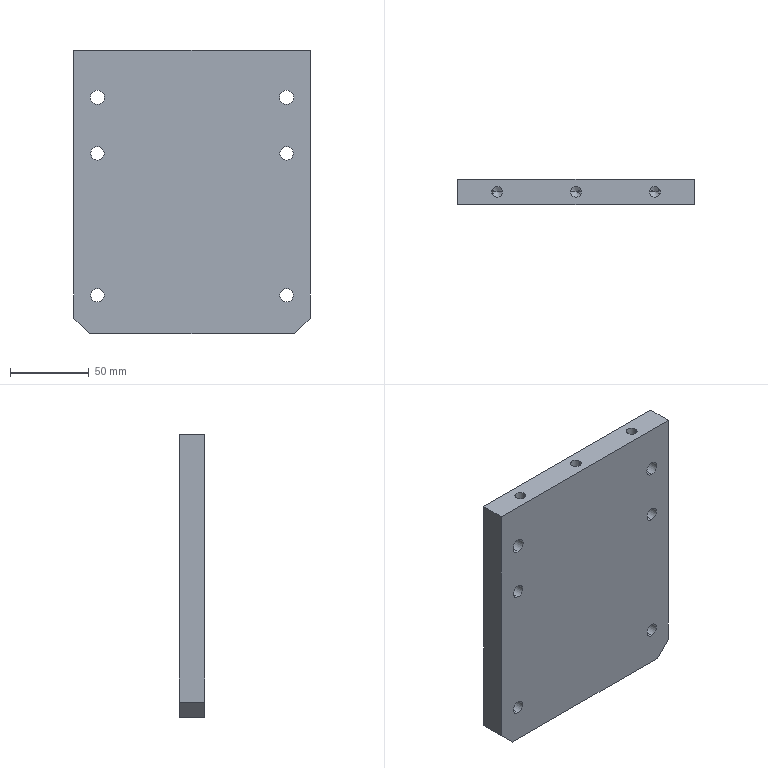Part | SolidWorks | features HoleWzd 3, Chamfer 1, Extrusion 1 | 1 solid | 38 faces | box 150 x 16 x 180 mm | volume 419444 mm3 | cylinder 22 | plane 10 | cone 6 | commonest cylinder face diameters 8.5 x8 6.8 x6 9 x4 15 x4
STEP:
#1=CARTESIAN_POINT('',(-60.,0.,-69.77));
#2=VERTEX_POINT('',#1);
#3=CARTESIAN_POINT('',(-60.,0.,-61.27));
#4=VERTEX_POINT('',#3);
#5=CARTESIAN_POINT('',(-60.,0.,-65.52));
#6=DIRECTION('',(0.,1.,0.));
#7=DIRECTION('',(0.,0.,1.));
#8=AXIS2_PLACEMENT_3D('',#5,#6,#7);
#9=CIRCLE('',#8,4.25);
#10=EDGE_CURVE('',#2,#4,#9,.T.);
#11=ORIENTED_EDGE('',*,*,#10,.F.);
#12=CARTESIAN_POINT('',(-60.,16.,-69.77));
#13=VERTEX_POINT('',#12);
#14=CARTESIAN_POINT('',(-60.,16.,-69.77));
#15=DIRECTION('',(0.,1.,0.));
#16=VECTOR('',#15,1000.);
#17=LINE('',#14,#16);
#18=EDGE_CURVE('',#2,#13,#17,.T.);
#19=ORIENTED_EDGE('',*,*,#18,.T.);
#20=CARTESIAN_POINT('',(-60.,16.,-61.27));
#21=VERTEX_POINT('',#20);
#22=CARTESIAN_POINT('',(-60.,16.,-65.52));
#23=DIRECTION('',(0.,1.,0.));
#24=DIRECTION('',(0.,0.,1.));
#25=AXIS2_PLACEMENT_3D('',#22,#23,#24);
#26=CIRCLE('',#25,4.25);
#27=EDGE_CURVE('',#13,#21,#26,.T.);
#28=ORIENTED_EDGE('',*,*,#27,.T.);
#29=CARTESIAN_POINT('',(-60.,16.,-61.27));
#30=DIRECTION('',(0.,1.,0.));
#31=VECTOR('',#30,1000.);
#32=LINE('',#29,#31);
#33=EDGE_CURVE('',#4,#21,#32,.T.);
#34=ORIENTED_EDGE('',*,*,#33,.F.);
#35=EDGE_LOOP('',(#11,#19,#28,#34));
#36=FACE_OUTER_BOUND('',#35,.T.);
#37=CARTESIAN_POINT('',(-60.,16.,-65.52));
#38=DIRECTION('',(0.,1.,0.));
#39=DIRECTION('',(0.,0.,1.));
#40=AXIS2_PLACEMENT_3D('',#37,#38,#39);
#41=CYLINDRICAL_SURFACE('',#40,4.25);
#42=ADVANCED_FACE('',(#36),#41,.F.);
#43=CARTESIAN_POINT('',(60.,0.,-69.77));
#44=VERTEX_POINT('',#43);
#45=CARTESIAN_POINT('',(60.,0.,-61.27));
#46=VERTEX_POINT('',#45);
#47=CARTESIAN_POINT('',(60.,0.,-65.52));
#48=DIRECTION('',(0.,1.,0.));
#49=DIRECTION('',(0.,0.,1.));
#50=AXIS2_PLACEMENT_3D('',#47,#48,#49);
#51=CIRCLE('',#50,4.25);
#52=EDGE_CURVE('',#44,#46,#51,.T.);
#53=ORIENTED_EDGE('',*,*,#52,.F.);
#54=CARTESIAN_POINT('',(60.,16.,-69.77));
#55=VERTEX_POINT('',#54);
#56=CARTESIAN_POINT('',(60.,16.,-69.77));
#57=DIRECTION('',(0.,1.,0.));
#58=VECTOR('',#57,1000.);
#59=LINE('',#56,#58);
#60=EDGE_CURVE('',#44,#55,#59,.T.);
#61=ORIENTED_EDGE('',*,*,#60,.T.);
#62=CARTESIAN_POINT('',(60.,16.,-61.27));
#63=VERTEX_POINT('',#62);
#64=CARTESIAN_POINT('',(60.,16.,-65.52));
#65=DIRECTION('',(0.,1.,0.));
#66=DIRECTION('',(0.,0.,1.));
#67=AXIS2_PLACEMENT_3D('',#64,#65,#66);
#68=CIRCLE('',#67,4.25);
#69=EDGE_CURVE('',#55,#63,#68,.T.);
#70=ORIENTED_EDGE('',*,*,#69,.T.);
#71=CARTESIAN_POINT('',(60.,16.,-61.27));
#72=DIRECTION('',(0.,1.,0.));
#73=VECTOR('',#72,1000.);
#74=LINE('',#71,#73);
#75=EDGE_CURVE('',#46,#63,#74,.T.);
#76=ORIENTED_EDGE('',*,*,#75,.F.);
#77=EDGE_LOOP('',(#53,#61,#70,#76));
#78=FACE_OUTER_BOUND('',#77,.T.);
#79=CARTESIAN_POINT('',(60.,16.,-65.52));
#80=DIRECTION('',(0.,1.,0.));
#81=DIRECTION('',(0.,0.,1.));
#82=AXIS2_PLACEMENT_3D('',#79,#80,#81);
#83=CYLINDRICAL_SURFACE('',#82,4.25);
#84=ADVANCED_FACE('',(#78),#83,.F.);
#85=CARTESIAN_POINT('',(-60.,0.,20.23));
#86=VERTEX_POINT('',#85);
#87=CARTESIAN_POINT('',(-60.,0.,28.73));
#88=VERTEX_POINT('',#87);
#89=CARTESIAN_POINT('',(-60.,0.,24.48));
#90=DIRECTION('',(0.,1.,0.));
#91=DIRECTION('',(0.,0.,1.));
#92=AXIS2_PLACEMENT_3D('',#89,#90,#91);
#93=CIRCLE('',#92,4.25);
#94=EDGE_CURVE('',#86,#88,#93,.T.);
#95=ORIENTED_EDGE('',*,*,#94,.F.);
#96=CARTESIAN_POINT('',(-60.,16.,20.23));
#97=VERTEX_POINT('',#96);
#98=CARTESIAN_POINT('',(-60.,16.,20.23));
#99=DIRECTION('',(0.,1.,0.));
#100=VECTOR('',#99,1000.);
#101=LINE('',#98,#100);
#102=EDGE_CURVE('',#86,#97,#101,.T.);
#103=ORIENTED_EDGE('',*,*,#102,.T.);
#104=CARTESIAN_POINT('',(-60.,16.,28.73));
#105=VERTEX_POINT('',#104);
#106=CARTESIAN_POINT('',(-60.,16.,24.48));
#107=DIRECTION('',(0.,1.,0.));
#108=DIRECTION('',(0.,0.,1.));
#109=AXIS2_PLACEMENT_3D('',#106,#107,#108);
#110=CIRCLE('',#109,4.25);
#111=EDGE_CURVE('',#97,#105,#110,.T.);
#112=ORIENTED_EDGE('',*,*,#111,.T.);
#113=CARTESIAN_POINT('',(-60.,16.,28.73));
#114=DIRECTION('',(0.,1.,0.));
#115=VECTOR('',#114,1000.);
#116=LINE('',#113,#115);
#117=EDGE_CURVE('',#88,#105,#116,.T.);
#118=ORIENTED_EDGE('',*,*,#117,.F.);
#119=EDGE_LOOP('',(#95,#103,#112,#118));
#120=FACE_OUTER_BOUND('',#119,.T.);
#121=CARTESIAN_POINT('',(-60.,16.,24.48));
#122=DIRECTION('',(0.,1.,0.));
#123=DIRECTION('',(0.,0.,1.));
#124=AXIS2_PLACEMENT_3D('',#121,#122,#123);
#125=CYLINDRICAL_SURFACE('',#124,4.25);
#126=ADVANCED_FACE('',(#120),#125,.F.);
#127=CARTESIAN_POINT('',(60.,0.,20.23));
#128=VERTEX_POINT('',#127);
#129=CARTESIAN_POINT('',(60.,0.,28.73));
#130=VERTEX_POINT('',#129);
#131=CARTESIAN_POINT('',(60.,0.,24.48));
#132=DIRECTION('',(0.,1.,0.));
#133=DIRECTION('',(0.,0.,1.));
#134=AXIS2_PLACEMENT_3D('',#131,#132,#133);
#135=CIRCLE('',#134,4.25);
#136=EDGE_CURVE('',#128,#130,#135,.T.);
#137=ORIENTED_EDGE('',*,*,#136,.F.);
#138=CARTESIAN_POINT('',(60.,16.,20.23));
#139=VERTEX_POINT('',#138);
#140=CARTESIAN_POINT('',(60.,16.,20.23));
#141=DIRECTION('',(0.,1.,0.));
#142=VECTOR('',#141,1000.);
#143=LINE('',#140,#142);
#144=EDGE_CURVE('',#128,#139,#143,.T.);
#145=ORIENTED_EDGE('',*,*,#144,.T.);
#146=CARTESIAN_POINT('',(60.,16.,28.73));
#147=VERTEX_POINT('',#146);
#148=CARTESIAN_POINT('',(60.,16.,24.48));
#149=DIRECTION('',(0.,1.,0.));
#150=DIRECTION('',(0.,0.,1.));
#151=AXIS2_PLACEMENT_3D('',#148,#149,#150);
#152=CIRCLE('',#151,4.25);
#153=EDGE_CURVE('',#139,#147,#152,.T.);
#154=ORIENTED_EDGE('',*,*,#153,.T.);
#155=CARTESIAN_POINT('',(60.,16.,28.73));
#156=DIRECTION('',(0.,1.,0.));
#157=VECTOR('',#156,1000.);
#158=LINE('',#155,#157);
#159=EDGE_CURVE('',#130,#147,#158,.T.);
#160=ORIENTED_EDGE('',*,*,#159,.F.);
#161=EDGE_LOOP('',(#137,#145,#154,#160));
#162=FACE_OUTER_BOUND('',#161,.T.);
#163=CARTESIAN_POINT('',(60.,16.,24.48));
#164=DIRECTION('',(0.,1.,0.));
#165=DIRECTION('',(0.,0.,1.));
#166=AXIS2_PLACEMENT_3D('',#163,#164,#165);
#167=CYLINDRICAL_SURFACE('',#166,4.25);
#168=ADVANCED_FACE('',(#162),#167,.F.);
#169=CARTESIAN_POINT('',(-60.,7.,52.5));
#170=VERTEX_POINT('',#169);
#171=CARTESIAN_POINT('',(-60.,7.,67.5));
#172=VERTEX_POINT('',#171);
#173=CARTESIAN_POINT('',(-60.,7.,60.));
#174=DIRECTION('',(0.,1.,0.));
#175=DIRECTION('',(0.,0.,1.));
#176=AXIS2_PLACEMENT_3D('',#173,#174,#175);
#177=CIRCLE('',#176,7.5);
#178=EDGE_CURVE('',#170,#172,#177,.T.);
#179=ORIENTED_EDGE('',*,*,#178,.F.);
#180=CARTESIAN_POINT('',(-60.,16.,52.5));
#181=VERTEX_POINT('',#180);
#182=CARTESIAN_POINT('',(-60.,16.,52.5));
#183=DIRECTION('',(0.,1.,0.));
#184=VECTOR('',#183,1000.);
#185=LINE('',#182,#184);
#186=EDGE_CURVE('',#170,#181,#185,.T.);
#187=ORIENTED_EDGE('',*,*,#186,.T.);
#188=CARTESIAN_POINT('',(-60.,16.,67.5));
#189=VERTEX_POINT('',#188);
#190=CARTESIAN_POINT('',(-60.,16.,60.));
#191=DIRECTION('',(0.,1.,0.));
#192=DIRECTION('',(0.,0.,1.));
#193=AXIS2_PLACEMENT_3D('',#190,#191,#192);
#194=CIRCLE('',#193,7.5);
#195=EDGE_CURVE('',#181,#189,#194,.T.);
#196=ORIENTED_EDGE('',*,*,#195,.T.);
#197=CARTESIAN_POINT('',(-60.,16.,67.5));
#198=DIRECTION('',(0.,1.,0.));
#199=VECTOR('',#198,1000.);
#200=LINE('',#197,#199);
#201=EDGE_CURVE('',#172,#189,#200,.T.);
#202=ORIENTED_EDGE('',*,*,#201,.F.);
#203=EDGE_LOOP('',(#179,#187,#196,#202));
#204=FACE_OUTER_BOUND('',#203,.T.);
#205=CARTESIAN_POINT('',(-60.,16.,60.));
#206=DIRECTION('',(0.,1.,0.));
#207=DIRECTION('',(0.,0.,1.));
#208=AXIS2_PLACEMENT_3D('',#205,#206,#207);
#209=CYLINDRICAL_SURFACE('',#208,7.5);
#210=ADVANCED_FACE('',(#204),#209,.F.);
#211=CARTESIAN_POINT('',(-60.,0.,55.5));
#212=VERTEX_POINT('',#211);
#213=CARTESIAN_POINT('',(-60.,0.,64.5));
#214=VERTEX_POINT('',#213);
#215=CARTESIAN_POINT('',(-60.,0.,60.));
#216=DIRECTION('',(0.,1.,0.));
#217=DIRECTION('',(0.,0.,1.));
#218=AXIS2_PLACEMENT_3D('',#215,#216,#217);
#219=CIRCLE('',#218,4.5);
#220=EDGE_CURVE('',#212,#214,#219,.T.);
#221=ORIENTED_EDGE('',*,*,#220,.F.);
#222=CARTESIAN_POINT('',(-60.,7.,55.5));
#223=VERTEX_POINT('',#222);
#224=CARTESIAN_POINT('',(-60.,16.,55.5));
#225=DIRECTION('',(0.,1.,0.));
#226=VECTOR('',#225,1000.);
#227=LINE('',#224,#226);
#228=EDGE_CURVE('',#212,#223,#227,.T.);
#229=ORIENTED_EDGE('',*,*,#228,.T.);
#230=CARTESIAN_POINT('',(-60.,7.,64.5));
#231=VERTEX_POINT('',#230);
#232=CARTESIAN_POINT('',(-60.,7.,60.));
#233=DIRECTION('',(0.,1.,0.));
#234=DIRECTION('',(0.,0.,1.));
#235=AXIS2_PLACEMENT_3D('',#232,#233,#234);
#236=CIRCLE('',#235,4.5);
#237=EDGE_CURVE('',#223,#231,#236,.T.);
#238=ORIENTED_EDGE('',*,*,#237,.T.);
#239=CARTESIAN_POINT('',(-60.,16.,64.5));
#240=DIRECTION('',(0.,1.,0.));
#241=VECTOR('',#240,1000.);
#242=LINE('',#239,#241);
#243=EDGE_CURVE('',#214,#231,#242,.T.);
#244=ORIENTED_EDGE('',*,*,#243,.F.);
#245=EDGE_LOOP('',(#221,#229,#238,#244));
#246=FACE_OUTER_BOUND('',#245,.T.);
#247=CARTESIAN_POINT('',(-60.,16.,60.));
#248=DIRECTION('',(0.,1.,0.));
#249=DIRECTION('',(0.,0.,1.));
#250=AXIS2_PLACEMENT_3D('',#247,#248,#249);
#251=CYLINDRICAL_SURFACE('',#250,4.5);
#252=ADVANCED_FACE('',(#246),#251,.F.);
#253=CARTESIAN_POINT('',(60.,7.,52.5));
#254=VERTEX_POINT('',#253);
#255=CARTESIAN_POINT('',(52.507,7.,60.329));
#256=VERTEX_POINT('',#255);
#257=CARTESIAN_POINT('',(60.,7.,60.));
#258=DIRECTION('',(0.,1.,0.));
#259=DIRECTION('',(0.,0.,1.));
#260=AXIS2_PLACEMENT_3D('',#257,#258,#259);
#261=CIRCLE('',#260,7.5);
#262=EDGE_CURVE('',#254,#256,#261,.T.);
#263=ORIENTED_EDGE('',*,*,#262,.F.);
#264=CARTESIAN_POINT('',(60.,16.,52.5));
#265=VERTEX_POINT('',#264);
#266=CARTESIAN_POINT('',(60.,16.,52.5));
#267=DIRECTION('',(0.,1.,0.));
#268=VECTOR('',#267,1000.);
#269=LINE('',#266,#268);
#270=EDGE_CURVE('',#254,#265,#269,.T.);
#271=ORIENTED_EDGE('',*,*,#270,.T.);
#272=CARTESIAN_POINT('',(60.,16.,67.5));
#273=VERTEX_POINT('',#272);
#274=CARTESIAN_POINT('',(60.,16.,60.));
#275=DIRECTION('',(0.,1.,0.));
#276=DIRECTION('',(0.,0.,1.));
#277=AXIS2_PLACEMENT_3D('',#274,#275,#276);
#278=CIRCLE('',#277,7.5);
#279=EDGE_CURVE('',#265,#273,#278,.T.);
#280=ORIENTED_EDGE('',*,*,#279,.T.);
#281=CARTESIAN_POINT('',(60.,7.,67.5));
#282=VERTEX_POINT('',#281);
#283=CARTESIAN_POINT('',(60.,16.,67.5));
#284=DIRECTION('',(0.,1.,0.));
#285=VECTOR('',#284,1000.);
#286=LINE('',#283,#285);
#287=EDGE_CURVE('',#282,#273,#286,.T.);
#288=ORIENTED_EDGE('',*,*,#287,.F.);
#289=CARTESIAN_POINT('',(53.25,7.,63.268));
#290=VERTEX_POINT('',#289);
#291=CARTESIAN_POINT('',(60.,7.,60.));
#292=DIRECTION('',(0.,1.,0.));
#293=DIRECTION('',(0.,0.,1.));
#294=AXIS2_PLACEMENT_3D('',#291,#292,#293);
#295=CIRCLE('',#294,7.5);
#296=EDGE_CURVE('',#290,#282,#295,.T.);
#297=ORIENTED_EDGE('',*,*,#296,.F.);
#298=CARTESIAN_POINT('',(53.4,8.,63.562));
#299=VERTEX_POINT('',#298);
#300=CARTESIAN_POINT('',(53.4,8.,63.562));
#301=CARTESIAN_POINT('',(53.4,7.823,63.562));
#302=CARTESIAN_POINT('',(53.386,7.644,63.536));
#303=CARTESIAN_POINT('',(53.333,7.307,63.436));
#304=CARTESIAN_POINT('',(53.295,7.147,63.362));
#305=CARTESIAN_POINT('',(53.25,7.,63.268));
#306=B_SPLINE_CURVE_WITH_KNOTS('',3,(#300,#301,#302,#303,#304,#305),.UNSPECIFIED.,.F.,.F.,(4,2,4),(0.004042,0.00457,0.005098),.UNSPECIFIED.);
#307=EDGE_CURVE('',#299,#290,#306,.T.);
#308=ORIENTED_EDGE('',*,*,#307,.F.);
#309=CARTESIAN_POINT('',(52.538,10.263,60.75));
#310=VERTEX_POINT('',#309);
#311=CARTESIAN_POINT('',(52.538,10.263,60.75));
#312=CARTESIAN_POINT('',(52.571,10.225,61.087));
#313=CARTESIAN_POINT('',(52.627,10.162,61.414));
#314=CARTESIAN_POINT('',(52.776,9.966,62.043));
#315=CARTESIAN_POINT('',(52.871,9.833,62.347));
#316=CARTESIAN_POINT('',(53.021,9.563,62.75));
#317=CARTESIAN_POINT('',(53.073,9.46,62.878));
#318=CARTESIAN_POINT('',(53.172,9.229,63.106));
#319=CARTESIAN_POINT('',(53.22,9.102,63.208));
#320=CARTESIAN_POINT('',(53.304,8.817,63.379));
#321=CARTESIAN_POINT('',(53.338,8.665,63.446));
#322=CARTESIAN_POINT('',(53.387,8.34,63.538));
#323=CARTESIAN_POINT('',(53.4,8.17,63.562));
#324=CARTESIAN_POINT('',(53.4,8.,63.562));
#325=B_SPLINE_CURVE_WITH_KNOTS('',3,(#311,#312,#313,#314,#315,#316,#317,#318,#319,#320,#321,#322,#323,#324),.UNSPECIFIED.,.F.,.F.,(4,2,2,2,2,2,4),(0.,0.001011,0.002021,0.002527,0.003032,0.003537,0.004042),.UNSPECIFIED.);
#326=EDGE_CURVE('',#310,#299,#325,.T.);
#327=ORIENTED_EDGE('',*,*,#326,.F.);
#328=CARTESIAN_POINT('',(52.503,8.,60.211));
#329=VERTEX_POINT('',#328);
#330=CARTESIAN_POINT('',(52.503,8.,60.211));
#331=CARTESIAN_POINT('',(52.503,8.196,60.211));
#332=CARTESIAN_POINT('',(52.503,8.393,60.225));
#333=CARTESIAN_POINT('',(52.505,8.778,60.279));
#334=CARTESIAN_POINT('',(52.507,8.968,60.318));
#335=CARTESIAN_POINT('',(52.514,9.533,60.464));
#336=CARTESIAN_POINT('',(52.522,9.902,60.599));
#337=CARTESIAN_POINT('',(52.538,10.263,60.75));
#338=B_SPLINE_CURVE_WITH_KNOTS('',3,(#330,#331,#332,#333,#334,#335,#336,#337),.UNSPECIFIED.,.F.,.F.,(4,2,2,4),(0.001459,0.002041,0.002623,0.003786),.UNSPECIFIED.);
#339=EDGE_CURVE('',#329,#310,#338,.T.);
#340=ORIENTED_EDGE('',*,*,#339,.F.);
#341=CARTESIAN_POINT('',(52.507,7.,60.329));
#342=CARTESIAN_POINT('',(52.504,7.328,60.254));
#343=CARTESIAN_POINT('',(52.503,7.661,60.211));
#344=CARTESIAN_POINT('',(52.503,8.,60.211));
#345=B_SPLINE_CURVE_WITH_KNOTS('',3,(#341,#342,#343,#344),.UNSPECIFIED.,.F.,.F.,(4,4),(0.000453,0.001459),.UNSPECIFIED.);
#346=EDGE_CURVE('',#256,#329,#345,.T.);
#347=ORIENTED_EDGE('',*,*,#346,.F.);
#348=EDGE_LOOP('',(#263,#271,#280,#288,#297,#308,#327,#340,#347));
#349=FACE_OUTER_BOUND('',#348,.T.);
#350=CARTESIAN_POINT('',(60.,16.,60.));
#351=DIRECTION('',(0.,1.,0.));
#352=DIRECTION('',(0.,0.,1.));
#353=AXIS2_PLACEMENT_3D('',#350,#351,#352);
#354=CYLINDRICAL_SURFACE('',#353,7.5);
#355=ADVANCED_FACE('',(#349),#354,.F.);
#356=CARTESIAN_POINT('',(60.,0.,55.5));
#357=VERTEX_POINT('',#356);
#358=CARTESIAN_POINT('',(60.,0.,64.5));
#359=VERTEX_POINT('',#358);
#360=CARTESIAN_POINT('',(60.,0.,60.));
#361=DIRECTION('',(0.,1.,0.));
#362=DIRECTION('',(0.,0.,1.));
#363=AXIS2_PLACEMENT_3D('',#360,#361,#362);
#364=CIRCLE('',#363,4.5);
#365=EDGE_CURVE('',#357,#359,#364,.T.);
#366=ORIENTED_EDGE('',*,*,#365,.F.);
#367=CARTESIAN_POINT('',(60.,7.,55.5));
#368=VERTEX_POINT('',#367);
#369=CARTESIAN_POINT('',(60.,16.,55.5));
#370=DIRECTION('',(0.,1.,0.));
#371=VECTOR('',#370,1000.);
#372=LINE('',#369,#371);
#373=EDGE_CURVE('',#357,#368,#372,.T.);
#374=ORIENTED_EDGE('',*,*,#373,.T.);
#375=CARTESIAN_POINT('',(60.,7.,64.5));
#376=VERTEX_POINT('',#375);
#377=CARTESIAN_POINT('',(60.,7.,60.));
#378=DIRECTION('',(0.,1.,0.));
#379=DIRECTION('',(0.,0.,1.));
#380=AXIS2_PLACEMENT_3D('',#377,#378,#379);
#381=CIRCLE('',#380,4.5);
#382=EDGE_CURVE('',#368,#376,#381,.T.);
#383=ORIENTED_EDGE('',*,*,#382,.T.);
#384=CARTESIAN_POINT('',(60.,16.,64.5));
#385=DIRECTION('',(0.,1.,0.));
#386=VECTOR('',#385,1000.);
#387=LINE('',#384,#386);
#388=EDGE_CURVE('',#359,#376,#387,.T.);
#389=ORIENTED_EDGE('',*,*,#388,.F.);
#390=EDGE_LOOP('',(#366,#374,#383,#389));
#391=FACE_OUTER_BOUND('',#390,.T.);
#392=CARTESIAN_POINT('',(60.,16.,60.));
#393=DIRECTION('',(0.,1.,0.));
#394=DIRECTION('',(0.,0.,1.));
#395=AXIS2_PLACEMENT_3D('',#392,#393,#394);
#396=CYLINDRICAL_SURFACE('',#395,4.5);
#397=ADVANCED_FACE('',(#391),#396,.F.);
#398=CARTESIAN_POINT('',(-53.25,7.,63.268));
#399=VERTEX_POINT('',#398);
#400=CARTESIAN_POINT('',(-53.4,8.,63.562));
#401=VERTEX_POINT('',#400);
#402=CARTESIAN_POINT('',(-53.25,7.,63.268));
#403=CARTESIAN_POINT('',(-53.295,7.147,63.362));
#404=CARTESIAN_POINT('',(-53.333,7.305,63.435));
#405=CARTESIAN_POINT('',(-53.386,7.645,63.536));
#406=CARTESIAN_POINT('',(-53.4,7.821,63.562));
#407=CARTESIAN_POINT('',(-53.4,8.,63.562));
#408=B_SPLINE_CURVE_WITH_KNOTS('',3,(#402,#403,#404,#405,#406,#407),.UNSPECIFIED.,.F.,.F.,(4,2,4),(0.,0.0005334,0.001067),.UNSPECIFIED.);
#409=EDGE_CURVE('',#399,#401,#408,.T.);
#410=ORIENTED_EDGE('',*,*,#409,.T.);
#411=CARTESIAN_POINT('',(-53.4,8.,90.));
#412=VERTEX_POINT('',#411);
#413=CARTESIAN_POINT('',(-53.4,8.,90.));
#414=DIRECTION('',(0.,0.,1.));
#415=VECTOR('',#414,1000.);
#416=LINE('',#413,#415);
#417=EDGE_CURVE('',#401,#412,#416,.T.);
#418=ORIENTED_EDGE('',*,*,#417,.T.);
#419=CARTESIAN_POINT('',(-46.6,8.,90.));
#420=VERTEX_POINT('',#419);
#421=CARTESIAN_POINT('',(-50.,8.,90.));
#422=DIRECTION('',(0.,0.,1.));
#423=DIRECTION('',(1.,0.,0.));
#424=AXIS2_PLACEMENT_3D('',#421,#422,#423);
#425=CIRCLE('',#424,3.4);
#426=EDGE_CURVE('',#412,#420,#425,.T.);
#427=ORIENTED_EDGE('',*,*,#426,.T.);
#428=CARTESIAN_POINT('',(-46.6,8.,60.75));
#429=VERTEX_POINT('',#428);
#430=CARTESIAN_POINT('',(-46.6,8.,90.));
#431=DIRECTION('',(0.,0.,1.));
#432=VECTOR('',#431,1000.);
#433=LINE('',#430,#432);
#434=EDGE_CURVE('',#429,#420,#433,.T.);
#435=ORIENTED_EDGE('',*,*,#434,.F.);
#436=CARTESIAN_POINT('',(-53.25,7.,60.75));
#437=VERTEX_POINT('',#436);
#438=CARTESIAN_POINT('',(-50.,8.,60.75));
#439=DIRECTION('',(0.,0.,1.));
#440=DIRECTION('',(1.,0.,0.));
#441=AXIS2_PLACEMENT_3D('',#438,#439,#440);
#442=CIRCLE('',#441,3.4);
#443=EDGE_CURVE('',#437,#429,#442,.T.);
#444=ORIENTED_EDGE('',*,*,#443,.F.);
#445=CARTESIAN_POINT('',(-53.25,7.,90.));
#446=DIRECTION('',(0.,0.,1.));
#447=VECTOR('',#446,1000.);
#448=LINE('',#445,#447);
#449=EDGE_CURVE('',#437,#399,#448,.T.);
#450=ORIENTED_EDGE('',*,*,#449,.T.);
#451=EDGE_LOOP('',(#410,#418,#427,#435,#444,#450));
#452=FACE_OUTER_BOUND('',#451,.T.);
#453=CARTESIAN_POINT('',(-50.,8.,90.));
#454=DIRECTION('',(0.,0.,1.));
#455=DIRECTION('',(1.,0.,0.));
#456=AXIS2_PLACEMENT_3D('',#453,#454,#455);
#457=CYLINDRICAL_SURFACE('',#456,3.4);
#458=ADVANCED_FACE('',(#452),#457,.F.);
#459=CARTESIAN_POINT('',(-50.,8.,58.707));
#460=VERTEX_POINT('',#459);
#461=CARTESIAN_POINT('',(-46.6,8.,60.75));
#462=DIRECTION('',(0.8572,0.,0.515));
#463=VECTOR('',#462,1000.);
#464=LINE('',#461,#463);
#465=EDGE_CURVE('',#460,#429,#464,.T.);
#466=ORIENTED_EDGE('',*,*,#465,.F.);
#467=CARTESIAN_POINT('',(-52.503,8.,60.211));
#468=VERTEX_POINT('',#467);
#469=CARTESIAN_POINT('',(-53.4,8.,60.75));
#470=DIRECTION('',(-0.8572,0.,0.515));
#471=VECTOR('',#470,1000.);
#472=LINE('',#469,#471);
#473=EDGE_CURVE('',#460,#468,#472,.T.);
#474=ORIENTED_EDGE('',*,*,#473,.T.);
#475=CARTESIAN_POINT('',(-52.507,7.,60.329));
#476=VERTEX_POINT('',#475);
#477=CARTESIAN_POINT('',(-52.503,8.,60.211));
#478=CARTESIAN_POINT('',(-52.503,7.665,60.211));
#479=CARTESIAN_POINT('',(-52.504,7.331,60.253));
#480=CARTESIAN_POINT('',(-52.507,7.,60.329));
#481=B_SPLINE_CURVE_WITH_KNOTS('',3,(#477,#478,#479,#480),.UNSPECIFIED.,.F.,.F.,(4,4),(0.002837,0.003843),.UNSPECIFIED.);
#482=EDGE_CURVE('',#468,#476,#481,.T.);
#483=ORIENTED_EDGE('',*,*,#482,.T.);
#484=CARTESIAN_POINT('',(-52.507,7.,60.329));
#485=CARTESIAN_POINT('',(-52.756,7.,60.468));
#486=CARTESIAN_POINT('',(-53.003,7.,60.608));
#487=CARTESIAN_POINT('',(-53.25,7.,60.75));
#488=B_SPLINE_CURVE_WITH_KNOTS('',3,(#484,#485,#486,#487),.UNSPECIFIED.,.F.,.F.,(4,4),(0.001162,0.002015),.UNSPECIFIED.);
#489=EDGE_CURVE('',#476,#437,#488,.T.);
#490=ORIENTED_EDGE('',*,*,#489,.T.);
#491=ORIENTED_EDGE('',*,*,#443,.T.);
#492=EDGE_LOOP('',(#466,#474,#483,#490,#491));
#493=FACE_OUTER_BOUND('',#492,.T.);
#494=CARTESIAN_POINT('',(-50.,8.,60.75));
#495=DIRECTION('',(0.,0.,1.));
#496=DIRECTION('',(1.,0.,0.));
#497=AXIS2_PLACEMENT_3D('',#494,#495,#496);
#498=CONICAL_SURFACE('',#497,3.4,1.03);
#499=ADVANCED_FACE('',(#493),#498,.F.);
#500=CARTESIAN_POINT('',(-3.4,8.,60.75));
#501=VERTEX_POINT('',#500);
#502=CARTESIAN_POINT('',(3.4,8.,60.75));
#503=VERTEX_POINT('',#502);
#504=CARTESIAN_POINT('',(0.,8.,60.75));
#505=DIRECTION('',(0.,0.,1.));
#506=DIRECTION('',(1.,0.,0.));
#507=AXIS2_PLACEMENT_3D('',#504,#505,#506);
#508=CIRCLE('',#507,3.4);
#509=EDGE_CURVE('',#501,#503,#508,.T.);
#510=ORIENTED_EDGE('',*,*,#509,.F.);
#511=CARTESIAN_POINT('',(-3.4,8.,90.));
#512=VERTEX_POINT('',#511);
#513=CARTESIAN_POINT('',(-3.4,8.,90.));
#514=DIRECTION('',(0.,0.,1.));
#515=VECTOR('',#514,1000.);
#516=LINE('',#513,#515);
#517=EDGE_CURVE('',#501,#512,#516,.T.);
#518=ORIENTED_EDGE('',*,*,#517,.T.);
#519=CARTESIAN_POINT('',(3.4,8.,90.));
#520=VERTEX_POINT('',#519);
#521=CARTESIAN_POINT('',(0.,8.,90.));
#522=DIRECTION('',(0.,0.,1.));
#523=DIRECTION('',(1.,0.,0.));
#524=AXIS2_PLACEMENT_3D('',#521,#522,#523);
#525=CIRCLE('',#524,3.4);
#526=EDGE_CURVE('',#512,#520,#525,.T.);
#527=ORIENTED_EDGE('',*,*,#526,.T.);
#528=CARTESIAN_POINT('',(3.4,8.,90.));
#529=DIRECTION('',(0.,0.,1.));
#530=VECTOR('',#529,1000.);
#531=LINE('',#528,#530);
#532=EDGE_CURVE('',#503,#520,#531,.T.);
#533=ORIENTED_EDGE('',*,*,#532,.F.);
#534=EDGE_LOOP('',(#510,#518,#527,#533));
#535=FACE_OUTER_BOUND('',#534,.T.);
#536=CARTESIAN_POINT('',(0.,8.,90.));
#537=DIRECTION('',(0.,0.,1.));
#538=DIRECTION('',(1.,0.,0.));
#539=AXIS2_PLACEMENT_3D('',#536,#537,#538);
#540=CYLINDRICAL_SURFACE('',#539,3.4);
#541=ADVANCED_FACE('',(#535),#540,.F.);
#542=CARTESIAN_POINT('',(0.,8.,58.707));
#543=VERTEX_POINT('',#542);
#544=CARTESIAN_POINT('',(3.4,8.,60.75));
#545=DIRECTION('',(0.8572,0.,0.515));
#546=VECTOR('',#545,1000.);
#547=LINE('',#544,#546);
#548=EDGE_CURVE('',#543,#503,#547,.T.);
#549=ORIENTED_EDGE('',*,*,#548,.F.);
#550=CARTESIAN_POINT('',(-3.4,8.,60.75));
#551=DIRECTION('',(-0.8572,0.,0.515));
#552=VECTOR('',#551,1000.);
#553=LINE('',#550,#552);
#554=EDGE_CURVE('',#543,#501,#553,.T.);
#555=ORIENTED_EDGE('',*,*,#554,.T.);
#556=ORIENTED_EDGE('',*,*,#509,.T.);
#557=EDGE_LOOP('',(#549,#555,#556));
#558=FACE_OUTER_BOUND('',#557,.T.);
#559=CARTESIAN_POINT('',(0.,8.,60.75));
#560=DIRECTION('',(0.,0.,1.));
#561=DIRECTION('',(1.,0.,0.));
#562=AXIS2_PLACEMENT_3D('',#559,#560,#561);
#563=CONICAL_SURFACE('',#562,3.4,1.03);
#564=ADVANCED_FACE('',(#558),#563,.F.);
#565=CARTESIAN_POINT('',(46.6,8.,60.75));
#566=VERTEX_POINT('',#565);
#567=CARTESIAN_POINT('',(53.25,7.,60.75));
#568=VERTEX_POINT('',#567);
#569=CARTESIAN_POINT('',(50.,8.,60.75));
#570=DIRECTION('',(0.,0.,1.));
#571=DIRECTION('',(1.,0.,0.));
#572=AXIS2_PLACEMENT_3D('',#569,#570,#571);
#573=CIRCLE('',#572,3.4);
#574=EDGE_CURVE('',#566,#568,#573,.T.);
#575=ORIENTED_EDGE('',*,*,#574,.F.);
#576=CARTESIAN_POINT('',(46.6,8.,90.));
#577=VERTEX_POINT('',#576);
#578=CARTESIAN_POINT('',(46.6,8.,90.));
#579=DIRECTION('',(0.,0.,1.));
#580=VECTOR('',#579,1000.);
#581=LINE('',#578,#580);
#582=EDGE_CURVE('',#566,#577,#581,.T.);
#583=ORIENTED_EDGE('',*,*,#582,.T.);
#584=CARTESIAN_POINT('',(53.4,8.,90.));
#585=VERTEX_POINT('',#584);
#586=CARTESIAN_POINT('',(50.,8.,90.));
#587=DIRECTION('',(0.,0.,1.));
#588=DIRECTION('',(1.,0.,0.));
#589=AXIS2_PLACEMENT_3D('',#586,#587,#588);
#590=CIRCLE('',#589,3.4);
#591=EDGE_CURVE('',#577,#585,#590,.T.);
#592=ORIENTED_EDGE('',*,*,#591,.T.);
#593=CARTESIAN_POINT('',(53.4,8.,90.));
#594=DIRECTION('',(0.,0.,1.));
#595=VECTOR('',#594,1000.);
#596=LINE('',#593,#595);
#597=EDGE_CURVE('',#299,#585,#596,.T.);
#598=ORIENTED_EDGE('',*,*,#597,.F.);
#599=ORIENTED_EDGE('',*,*,#307,.T.);
#600=CARTESIAN_POINT('',(53.25,7.,90.));
#601=DIRECTION('',(0.,0.,-1.));
#602=VECTOR('',#601,1000.);
#603=LINE('',#600,#602);
#604=EDGE_CURVE('',#290,#568,#603,.T.);
#605=ORIENTED_EDGE('',*,*,#604,.T.);
#606=EDGE_LOOP('',(#575,#583,#592,#598,#599,#605));
#607=FACE_OUTER_BOUND('',#606,.T.);
#608=CARTESIAN_POINT('',(50.,8.,90.));
#609=DIRECTION('',(0.,0.,1.));
#610=DIRECTION('',(1.,0.,0.));
#611=AXIS2_PLACEMENT_3D('',#608,#609,#610);
#612=CYLINDRICAL_SURFACE('',#611,3.4);
#613=ADVANCED_FACE('',(#607),#612,.F.);
#614=CARTESIAN_POINT('',(50.,8.,58.707));
#615=VERTEX_POINT('',#614);
#616=CARTESIAN_POINT('',(53.4,8.,60.75));
#617=DIRECTION('',(0.8572,0.,0.515));
#618=VECTOR('',#617,1000.);
#619=LINE('',#616,#618);
#620=EDGE_CURVE('',#615,#329,#619,.T.);
#621=ORIENTED_EDGE('',*,*,#620,.F.);
#622=CARTESIAN_POINT('',(46.6,8.,60.75));
#623=DIRECTION('',(-0.8572,0.,0.515));
#624=VECTOR('',#623,1000.);
#625=LINE('',#622,#624);
#626=EDGE_CURVE('',#615,#566,#625,.T.);
#627=ORIENTED_EDGE('',*,*,#626,.T.);
#628=ORIENTED_EDGE('',*,*,#574,.T.);
#629=CARTESIAN_POINT('',(53.25,7.,60.75));
#630=CARTESIAN_POINT('',(53.003,7.,60.608));
#631=CARTESIAN_POINT('',(52.756,7.,60.468));
#632=CARTESIAN_POINT('',(52.507,7.,60.329));
#633=B_SPLINE_CURVE_WITH_KNOTS('',3,(#629,#630,#631,#632),.UNSPECIFIED.,.F.,.F.,(4,4),(0.002563,0.003416),.UNSPECIFIED.);
#634=EDGE_CURVE('',#568,#256,#633,.T.);
#635=ORIENTED_EDGE('',*,*,#634,.T.);
#636=ORIENTED_EDGE('',*,*,#346,.T.);
#637=EDGE_LOOP('',(#621,#627,#628,#635,#636));
#638=FACE_OUTER_BOUND('',#637,.T.);
#639=CARTESIAN_POINT('',(50.,8.,60.75));
#640=DIRECTION('',(0.,0.,1.));
#641=DIRECTION('',(1.,0.,0.));
#642=AXIS2_PLACEMENT_3D('',#639,#640,#641);
#643=CONICAL_SURFACE('',#642,3.4,1.03);
#644=ADVANCED_FACE('',(#638),#643,.F.);
#645=CARTESIAN_POINT('',(75.,0.,90.));
#646=VERTEX_POINT('',#645);
#647=CARTESIAN_POINT('',(75.,0.,-80.));
#648=VERTEX_POINT('',#647);
#649=CARTESIAN_POINT('',(75.,0.,-90.));
#650=DIRECTION('',(0.,0.,-1.));
#651=VECTOR('',#650,1000.);
#652=LINE('',#649,#651);
#653=EDGE_CURVE('',#646,#648,#652,.T.);
#654=ORIENTED_EDGE('',*,*,#653,.T.);
#655=CARTESIAN_POINT('',(75.,16.,-80.));
#656=VERTEX_POINT('',#655);
#657=CARTESIAN_POINT('',(75.,16.,-80.));
#658=DIRECTION('',(0.,1.,0.));
#659=VECTOR('',#658,1000.);
#660=LINE('',#657,#659);
#661=EDGE_CURVE('',#648,#656,#660,.T.);
#662=ORIENTED_EDGE('',*,*,#661,.T.);
#663=CARTESIAN_POINT('',(75.,16.,90.));
#664=VERTEX_POINT('',#663);
#665=CARTESIAN_POINT('',(75.,16.,-90.));
#666=DIRECTION('',(0.,0.,-1.));
#667=VECTOR('',#666,1000.);
#668=LINE('',#665,#667);
#669=EDGE_CURVE('',#664,#656,#668,.T.);
#670=ORIENTED_EDGE('',*,*,#669,.F.);
#671=CARTESIAN_POINT('',(75.,16.,90.));
#672=DIRECTION('',(0.,-1.,0.));
#673=VECTOR('',#672,1000.);
#674=LINE('',#671,#673);
#675=EDGE_CURVE('',#664,#646,#674,.T.);
#676=ORIENTED_EDGE('',*,*,#675,.T.);
#677=EDGE_LOOP('',(#654,#662,#670,#676));
#678=FACE_OUTER_BOUND('',#677,.T.);
#679=CARTESIAN_POINT('',(75.,16.,-90.));
#680=DIRECTION('',(-1.,0.,0.));
#681=DIRECTION('',(0.,0.,1.));
#682=AXIS2_PLACEMENT_3D('',#679,#680,#681);
#683=PLANE('',#682);
#684=ADVANCED_FACE('',(#678),#683,.F.);
#685=CARTESIAN_POINT('',(65.,0.,-90.));
#686=VERTEX_POINT('',#685);
#687=CARTESIAN_POINT('',(-65.,0.,-90.));
#688=VERTEX_POINT('',#687);
#689=CARTESIAN_POINT('',(-75.,0.,-90.));
#690=DIRECTION('',(-1.,0.,0.));
#691=VECTOR('',#690,1000.);
#692=LINE('',#689,#691);
#693=EDGE_CURVE('',#686,#688,#692,.T.);
#694=ORIENTED_EDGE('',*,*,#693,.T.);
#695=CARTESIAN_POINT('',(-65.,16.,-90.));
#696=VERTEX_POINT('',#695);
#697=CARTESIAN_POINT('',(-65.,16.,-90.));
#698=DIRECTION('',(0.,1.,0.));
#699=VECTOR('',#698,1000.);
#700=LINE('',#697,#699);
#701=EDGE_CURVE('',#688,#696,#700,.T.);
#702=ORIENTED_EDGE('',*,*,#701,.T.);
#703=CARTESIAN_POINT('',(65.,16.,-90.));
#704=VERTEX_POINT('',#703);
#705=CARTESIAN_POINT('',(-75.,16.,-90.));
#706=DIRECTION('',(-1.,0.,0.));
#707=VECTOR('',#706,1000.);
#708=LINE('',#705,#707);
#709=EDGE_CURVE('',#704,#696,#708,.T.);
#710=ORIENTED_EDGE('',*,*,#709,.F.);
#711=CARTESIAN_POINT('',(65.,16.,-90.));
#712=DIRECTION('',(0.,-1.,0.));
#713=VECTOR('',#712,1000.);
#714=LINE('',#711,#713);
#715=EDGE_CURVE('',#704,#686,#714,.T.);
#716=ORIENTED_EDGE('',*,*,#715,.T.);
#717=EDGE_LOOP('',(#694,#702,#710,#716));
#718=FACE_OUTER_BOUND('',#717,.T.);
#719=CARTESIAN_POINT('',(-75.,16.,-90.));
#720=DIRECTION('',(0.,0.,1.));
#721=DIRECTION('',(1.,0.,0.));
#722=AXIS2_PLACEMENT_3D('',#719,#720,#721);
#723=PLANE('',#722);
#724=ADVANCED_FACE('',(#718),#723,.F.);
#725=CARTESIAN_POINT('',(-75.,16.,-80.));
#726=VERTEX_POINT('',#725);
#727=CARTESIAN_POINT('',(-75.,16.,90.));
#728=VERTEX_POINT('',#727);
#729=CARTESIAN_POINT('',(-75.,16.,-90.));
#730=DIRECTION('',(0.,0.,1.));
#731=VECTOR('',#730,1000.);
#732=LINE('',#729,#731);
#733=EDGE_CURVE('',#726,#728,#732,.T.);
#734=ORIENTED_EDGE('',*,*,#733,.F.);
#735=CARTESIAN_POINT('',(-75.,0.,-80.));
#736=VERTEX_POINT('',#735);
#737=CARTESIAN_POINT('',(-75.,16.,-80.));
#738=DIRECTION('',(0.,-1.,0.));
#739=VECTOR('',#738,1000.);
#740=LINE('',#737,#739);
#741=EDGE_CURVE('',#726,#736,#740,.T.);
#742=ORIENTED_EDGE('',*,*,#741,.T.);
#743=CARTESIAN_POINT('',(-75.,0.,90.));
#744=VERTEX_POINT('',#743);
#745=CARTESIAN_POINT('',(-75.,0.,-90.));
#746=DIRECTION('',(0.,0.,1.));
#747=VECTOR('',#746,1000.);
#748=LINE('',#745,#747);
#749=EDGE_CURVE('',#736,#744,#748,.T.);
#750=ORIENTED_EDGE('',*,*,#749,.T.);
#751=CARTESIAN_POINT('',(-75.,16.,90.));
#752=DIRECTION('',(0.,-1.,0.));
#753=VECTOR('',#752,1000.);
#754=LINE('',#751,#753);
#755=EDGE_CURVE('',#728,#744,#754,.T.);
#756=ORIENTED_EDGE('',*,*,#755,.F.);
#757=EDGE_LOOP('',(#734,#742,#750,#756));
#758=FACE_OUTER_BOUND('',#757,.T.);
#759=CARTESIAN_POINT('',(-75.,16.,-90.));
#760=DIRECTION('',(1.,0.,0.));
#761=DIRECTION('',(0.,0.,-1.));
#762=AXIS2_PLACEMENT_3D('',#759,#760,#761);
#763=PLANE('',#762);
#764=ADVANCED_FACE('',(#758),#763,.F.);
#765=CARTESIAN_POINT('',(-50.,8.,90.));
#766=DIRECTION('',(0.,0.,1.));
#767=DIRECTION('',(1.,0.,0.));
#768=AXIS2_PLACEMENT_3D('',#765,#766,#767);
#769=CIRCLE('',#768,3.4);
#770=EDGE_CURVE('',#420,#412,#769,.T.);
#771=ORIENTED_EDGE('',*,*,#770,.F.);
#772=ORIENTED_EDGE('',*,*,#426,.F.);
#773=EDGE_LOOP('',(#771,#772));
#774=FACE_BOUND('',#773,.T.);
#775=CARTESIAN_POINT('',(0.,8.,90.));
#776=DIRECTION('',(0.,0.,1.));
#777=DIRECTION('',(1.,0.,0.));
#778=AXIS2_PLACEMENT_3D('',#775,#776,#777);
#779=CIRCLE('',#778,3.4);
#780=EDGE_CURVE('',#520,#512,#779,.T.);
#781=ORIENTED_EDGE('',*,*,#780,.F.);
#782=ORIENTED_EDGE('',*,*,#526,.F.);
#783=EDGE_LOOP('',(#781,#782));
#784=FACE_BOUND('',#783,.T.);
#785=CARTESIAN_POINT('',(50.,8.,90.));
#786=DIRECTION('',(0.,0.,1.));
#787=DIRECTION('',(1.,0.,0.));
#788=AXIS2_PLACEMENT_3D('',#785,#786,#787);
#789=CIRCLE('',#788,3.4);
#790=EDGE_CURVE('',#585,#577,#789,.T.);
#791=ORIENTED_EDGE('',*,*,#790,.F.);
#792=ORIENTED_EDGE('',*,*,#591,.F.);
#793=EDGE_LOOP('',(#791,#792));
#794=FACE_BOUND('',#793,.T.);
#795=CARTESIAN_POINT('',(-75.,0.,90.));
#796=DIRECTION('',(1.,0.,0.));
#797=VECTOR('',#796,1000.);
#798=LINE('',#795,#797);
#799=EDGE_CURVE('',#744,#646,#798,.T.);
#800=ORIENTED_EDGE('',*,*,#799,.T.);
#801=ORIENTED_EDGE('',*,*,#675,.F.);
#802=CARTESIAN_POINT('',(-75.,16.,90.));
#803=DIRECTION('',(1.,0.,0.));
#804=VECTOR('',#803,1000.);
#805=LINE('',#802,#804);
#806=EDGE_CURVE('',#728,#664,#805,.T.);
#807=ORIENTED_EDGE('',*,*,#806,.F.);
#808=ORIENTED_EDGE('',*,*,#755,.T.);
#809=EDGE_LOOP('',(#800,#801,#807,#808));
#810=FACE_OUTER_BOUND('',#809,.T.);
#811=CARTESIAN_POINT('',(-75.,16.,90.));
#812=DIRECTION('',(0.,0.,-1.));
#813=DIRECTION('',(-1.,0.,0.));
#814=AXIS2_PLACEMENT_3D('',#811,#812,#813);
#815=PLANE('',#814);
#816=ADVANCED_FACE('',(#774,#784,#794,#810),#815,.F.);
#817=CARTESIAN_POINT('',(-60.,16.,-65.52));
#818=DIRECTION('',(0.,1.,0.));
#819=DIRECTION('',(0.,0.,1.));
#820=AXIS2_PLACEMENT_3D('',#817,#818,#819);
#821=CIRCLE('',#820,4.25);
#822=EDGE_CURVE('',#21,#13,#821,.T.);
#823=ORIENTED_EDGE('',*,*,#822,.F.);
#824=ORIENTED_EDGE('',*,*,#27,.F.);
#825=EDGE_LOOP('',(#823,#824));
#826=FACE_BOUND('',#825,.T.);
#827=CARTESIAN_POINT('',(60.,16.,-65.52));
#828=DIRECTION('',(0.,1.,0.));
#829=DIRECTION('',(0.,0.,1.));
#830=AXIS2_PLACEMENT_3D('',#827,#828,#829);
#831=CIRCLE('',#830,4.25);
#832=EDGE_CURVE('',#63,#55,#831,.T.);
#833=ORIENTED_EDGE('',*,*,#832,.F.);
#834=ORIENTED_EDGE('',*,*,#69,.F.);
#835=EDGE_LOOP('',(#833,#834));
#836=FACE_BOUND('',#835,.T.);
#837=CARTESIAN_POINT('',(-60.,16.,24.48));
#838=DIRECTION('',(0.,1.,0.));
#839=DIRECTION('',(0.,0.,1.));
#840=AXIS2_PLACEMENT_3D('',#837,#838,#839);
#841=CIRCLE('',#840,4.25);
#842=EDGE_CURVE('',#105,#97,#841,.T.);
#843=ORIENTED_EDGE('',*,*,#842,.F.);
#844=ORIENTED_EDGE('',*,*,#111,.F.);
#845=EDGE_LOOP('',(#843,#844));
#846=FACE_BOUND('',#845,.T.);
#847=CARTESIAN_POINT('',(60.,16.,24.48));
#848=DIRECTION('',(0.,1.,0.));
#849=DIRECTION('',(0.,0.,1.));
#850=AXIS2_PLACEMENT_3D('',#847,#848,#849);
#851=CIRCLE('',#850,4.25);
#852=EDGE_CURVE('',#147,#139,#851,.T.);
#853=ORIENTED_EDGE('',*,*,#852,.F.);
#854=ORIENTED_EDGE('',*,*,#153,.F.);
#855=EDGE_LOOP('',(#853,#854));
#856=FACE_BOUND('',#855,.T.);
#857=CARTESIAN_POINT('',(-60.,16.,60.));
#858=DIRECTION('',(0.,1.,0.));
#859=DIRECTION('',(0.,0.,1.));
#860=AXIS2_PLACEMENT_3D('',#857,#858,#859);
#861=CIRCLE('',#860,7.5);
#862=EDGE_CURVE('',#189,#181,#861,.T.);
#863=ORIENTED_EDGE('',*,*,#862,.F.);
#864=ORIENTED_EDGE('',*,*,#195,.F.);
#865=EDGE_LOOP('',(#863,#864));
#866=FACE_BOUND('',#865,.T.);
#867=CARTESIAN_POINT('',(60.,16.,60.));
#868=DIRECTION('',(0.,1.,0.));
#869=DIRECTION('',(0.,0.,1.));
#870=AXIS2_PLACEMENT_3D('',#867,#868,#869);
#871=CIRCLE('',#870,7.5);
#872=EDGE_CURVE('',#273,#265,#871,.T.);
#873=ORIENTED_EDGE('',*,*,#872,.F.);
#874=ORIENTED_EDGE('',*,*,#279,.F.);
#875=EDGE_LOOP('',(#873,#874));
#876=FACE_BOUND('',#875,.T.);
#877=ORIENTED_EDGE('',*,*,#709,.T.);
#878=CARTESIAN_POINT('',(-77.5,16.,-77.5));
#879=DIRECTION('',(-0.7071,0.,0.7071));
#880=VECTOR('',#879,1000.);
#881=LINE('',#878,#880);
#882=EDGE_CURVE('',#696,#726,#881,.T.);
#883=ORIENTED_EDGE('',*,*,#882,.T.);
#884=ORIENTED_EDGE('',*,*,#733,.T.);
#885=ORIENTED_EDGE('',*,*,#806,.T.);
#886=ORIENTED_EDGE('',*,*,#669,.T.);
#887=CARTESIAN_POINT('',(77.5,16.,-77.5));
#888=DIRECTION('',(-0.7071,0.,-0.7071));
#889=VECTOR('',#888,1000.);
#890=LINE('',#887,#889);
#891=EDGE_CURVE('',#656,#704,#890,.T.);
#892=ORIENTED_EDGE('',*,*,#891,.T.);
#893=EDGE_LOOP('',(#877,#883,#884,#885,#886,#892));
#894=FACE_OUTER_BOUND('',#893,.T.);
#895=CARTESIAN_POINT('',(0.,16.,0.));
#896=DIRECTION('',(0.,1.,0.));
#897=DIRECTION('',(0.,0.,1.));
#898=AXIS2_PLACEMENT_3D('',#895,#896,#897);
#899=PLANE('',#898);
#900=ADVANCED_FACE('',(#826,#836,#846,#856,#866,#876,#894),#899,.T.);
#901=CARTESIAN_POINT('',(-60.,0.,-65.52));
#902=DIRECTION('',(0.,1.,0.));
#903=DIRECTION('',(0.,0.,1.));
#904=AXIS2_PLACEMENT_3D('',#901,#902,#903);
#905=CIRCLE('',#904,4.25);
#906=EDGE_CURVE('',#4,#2,#905,.T.);
#907=ORIENTED_EDGE('',*,*,#906,.T.);
#908=ORIENTED_EDGE('',*,*,#10,.T.);
#909=EDGE_LOOP('',(#907,#908));
#910=FACE_BOUND('',#909,.T.);
#911=CARTESIAN_POINT('',(60.,0.,-65.52));
#912=DIRECTION('',(0.,1.,0.));
#913=DIRECTION('',(0.,0.,1.));
#914=AXIS2_PLACEMENT_3D('',#911,#912,#913);
#915=CIRCLE('',#914,4.25);
#916=EDGE_CURVE('',#46,#44,#915,.T.);
#917=ORIENTED_EDGE('',*,*,#916,.T.);
#918=ORIENTED_EDGE('',*,*,#52,.T.);
#919=EDGE_LOOP('',(#917,#918));
#920=FACE_BOUND('',#919,.T.);
#921=CARTESIAN_POINT('',(-60.,0.,24.48));
#922=DIRECTION('',(0.,1.,0.));
#923=DIRECTION('',(0.,0.,1.));
#924=AXIS2_PLACEMENT_3D('',#921,#922,#923);
#925=CIRCLE('',#924,4.25);
#926=EDGE_CURVE('',#88,#86,#925,.T.);
#927=ORIENTED_EDGE('',*,*,#926,.T.);
#928=ORIENTED_EDGE('',*,*,#94,.T.);
#929=EDGE_LOOP('',(#927,#928));
#930=FACE_BOUND('',#929,.T.);
#931=CARTESIAN_POINT('',(60.,0.,24.48));
#932=DIRECTION('',(0.,1.,0.));
#933=DIRECTION('',(0.,0.,1.));
#934=AXIS2_PLACEMENT_3D('',#931,#932,#933);
#935=CIRCLE('',#934,4.25);
#936=EDGE_CURVE('',#130,#128,#935,.T.);
#937=ORIENTED_EDGE('',*,*,#936,.T.);
#938=ORIENTED_EDGE('',*,*,#136,.T.);
#939=EDGE_LOOP('',(#937,#938));
#940=FACE_BOUND('',#939,.T.);
#941=CARTESIAN_POINT('',(-60.,0.,60.));
#942=DIRECTION('',(0.,1.,0.));
#943=DIRECTION('',(0.,0.,1.));
#944=AXIS2_PLACEMENT_3D('',#941,#942,#943);
#945=CIRCLE('',#944,4.5);
#946=EDGE_CURVE('',#214,#212,#945,.T.);
#947=ORIENTED_EDGE('',*,*,#946,.T.);
#948=ORIENTED_EDGE('',*,*,#220,.T.);
#949=EDGE_LOOP('',(#947,#948));
#950=FACE_BOUND('',#949,.T.);
#951=CARTESIAN_POINT('',(60.,0.,60.));
#952=DIRECTION('',(0.,1.,0.));
#953=DIRECTION('',(0.,0.,1.));
#954=AXIS2_PLACEMENT_3D('',#951,#952,#953);
#955=CIRCLE('',#954,4.5);
#956=EDGE_CURVE('',#359,#357,#955,.T.);
#957=ORIENTED_EDGE('',*,*,#956,.T.);
#958=ORIENTED_EDGE('',*,*,#365,.T.);
#959=EDGE_LOOP('',(#957,#958));
#960=FACE_BOUND('',#959,.T.);
#961=ORIENTED_EDGE('',*,*,#749,.F.);
#962=CARTESIAN_POINT('',(-75.,0.,-80.));
#963=DIRECTION('',(0.7071,0.,-0.7071));
#964=VECTOR('',#963,1000.);
#965=LINE('',#962,#964);
#966=EDGE_CURVE('',#736,#688,#965,.T.);
#967=ORIENTED_EDGE('',*,*,#966,.T.);
#968=ORIENTED_EDGE('',*,*,#693,.F.);
#969=CARTESIAN_POINT('',(65.,0.,-90.));
#970=DIRECTION('',(0.7071,0.,0.7071));
#971=VECTOR('',#970,1000.);
#972=LINE('',#969,#971);
#973=EDGE_CURVE('',#686,#648,#972,.T.);
#974=ORIENTED_EDGE('',*,*,#973,.T.);
#975=ORIENTED_EDGE('',*,*,#653,.F.);
#976=ORIENTED_EDGE('',*,*,#799,.F.);
#977=EDGE_LOOP('',(#961,#967,#968,#974,#975,#976));
#978=FACE_OUTER_BOUND('',#977,.T.);
#979=CARTESIAN_POINT('',(0.,0.,0.));
#980=DIRECTION('',(0.,1.,0.));
#981=DIRECTION('',(0.,0.,1.));
#982=AXIS2_PLACEMENT_3D('',#979,#980,#981);
#983=PLANE('',#982);
#984=ADVANCED_FACE('',(#910,#920,#930,#940,#950,#960,#978),#983,.F.);
#985=ORIENTED_EDGE('',*,*,#626,.F.);
#986=ORIENTED_EDGE('',*,*,#620,.T.);
#987=ORIENTED_EDGE('',*,*,#339,.T.);
#988=CARTESIAN_POINT('',(50.,8.,60.75));
#989=DIRECTION('',(0.,0.,1.));
#990=DIRECTION('',(1.,0.,0.));
#991=AXIS2_PLACEMENT_3D('',#988,#989,#990);
#992=CIRCLE('',#991,3.4);
#993=EDGE_CURVE('',#310,#566,#992,.T.);
#994=ORIENTED_EDGE('',*,*,#993,.T.);
#995=EDGE_LOOP('',(#985,#986,#987,#994));
#996=FACE_OUTER_BOUND('',#995,.T.);
#997=CARTESIAN_POINT('',(50.,8.,60.75));
#998=DIRECTION('',(0.,0.,1.));
#999=DIRECTION('',(1.,0.,0.));
#1000=AXIS2_PLACEMENT_3D('',#997,#998,#999);
#1001=CONICAL_SURFACE('',#1000,3.4,1.03);
#1002=ADVANCED_FACE('',(#996),#1001,.F.);
#1003=ORIENTED_EDGE('',*,*,#582,.F.);
#1004=ORIENTED_EDGE('',*,*,#993,.F.);
#1005=ORIENTED_EDGE('',*,*,#326,.T.);
#1006=ORIENTED_EDGE('',*,*,#597,.T.);
#1007=ORIENTED_EDGE('',*,*,#790,.T.);
#1008=EDGE_LOOP('',(#1003,#1004,#1005,#1006,#1007));
#1009=FACE_OUTER_BOUND('',#1008,.T.);
#1010=CARTESIAN_POINT('',(50.,8.,90.));
#1011=DIRECTION('',(0.,0.,1.));
#1012=DIRECTION('',(1.,0.,0.));
#1013=AXIS2_PLACEMENT_3D('',#1010,#1011,#1012);
#1014=CYLINDRICAL_SURFACE('',#1013,3.4);
#1015=ADVANCED_FACE('',(#1009),#1014,.F.);
#1016=ORIENTED_EDGE('',*,*,#554,.F.);
#1017=ORIENTED_EDGE('',*,*,#548,.T.);
#1018=CARTESIAN_POINT('',(0.,8.,60.75));
#1019=DIRECTION('',(0.,0.,1.));
#1020=DIRECTION('',(1.,0.,0.));
#1021=AXIS2_PLACEMENT_3D('',#1018,#1019,#1020);
#1022=CIRCLE('',#1021,3.4);
#1023=EDGE_CURVE('',#503,#501,#1022,.T.);
#1024=ORIENTED_EDGE('',*,*,#1023,.T.);
#1025=EDGE_LOOP('',(#1016,#1017,#1024));
#1026=FACE_OUTER_BOUND('',#1025,.T.);
#1027=CARTESIAN_POINT('',(0.,8.,60.75));
#1028=DIRECTION('',(0.,0.,1.));
#1029=DIRECTION('',(1.,0.,0.));
#1030=AXIS2_PLACEMENT_3D('',#1027,#1028,#1029);
#1031=CONICAL_SURFACE('',#1030,3.4,1.03);
#1032=ADVANCED_FACE('',(#1026),#1031,.F.);
#1033=ORIENTED_EDGE('',*,*,#517,.F.);
#1034=ORIENTED_EDGE('',*,*,#1023,.F.);
#1035=ORIENTED_EDGE('',*,*,#532,.T.);
#1036=ORIENTED_EDGE('',*,*,#780,.T.);
#1037=EDGE_LOOP('',(#1033,#1034,#1035,#1036));
#1038=FACE_OUTER_BOUND('',#1037,.T.);
#1039=CARTESIAN_POINT('',(0.,8.,90.));
#1040=DIRECTION('',(0.,0.,1.));
#1041=DIRECTION('',(1.,0.,0.));
#1042=AXIS2_PLACEMENT_3D('',#1039,#1040,#1041);
#1043=CYLINDRICAL_SURFACE('',#1042,3.4);
#1044=ADVANCED_FACE('',(#1038),#1043,.F.);
#1045=ORIENTED_EDGE('',*,*,#473,.F.);
#1046=ORIENTED_EDGE('',*,*,#465,.T.);
#1047=CARTESIAN_POINT('',(-52.538,10.263,60.75));
#1048=VERTEX_POINT('',#1047);
#1049=CARTESIAN_POINT('',(-50.,8.,60.75));
#1050=DIRECTION('',(0.,0.,1.));
#1051=DIRECTION('',(1.,0.,0.));
#1052=AXIS2_PLACEMENT_3D('',#1049,#1050,#1051);
#1053=CIRCLE('',#1052,3.4);
#1054=EDGE_CURVE('',#429,#1048,#1053,.T.);
#1055=ORIENTED_EDGE('',*,*,#1054,.T.);
#1056=CARTESIAN_POINT('',(-52.538,10.263,60.75));
#1057=CARTESIAN_POINT('',(-52.522,9.903,60.599));
#1058=CARTESIAN_POINT('',(-52.514,9.538,60.466));
#1059=CARTESIAN_POINT('',(-52.504,8.784,60.27));
#1060=CARTESIAN_POINT('',(-52.503,8.389,60.211));
#1061=CARTESIAN_POINT('',(-52.503,8.,60.211));
#1062=B_SPLINE_CURVE_WITH_KNOTS('',3,(#1056,#1057,#1058,#1059,#1060,#1061),.UNSPECIFIED.,.F.,.F.,(4,2,4),(0.0005043,0.001671,0.002837),.UNSPECIFIED.);
#1063=EDGE_CURVE('',#1048,#468,#1062,.T.);
#1064=ORIENTED_EDGE('',*,*,#1063,.T.);
#1065=EDGE_LOOP('',(#1045,#1046,#1055,#1064));
#1066=FACE_OUTER_BOUND('',#1065,.T.);
#1067=CARTESIAN_POINT('',(-50.,8.,60.75));
#1068=DIRECTION('',(0.,0.,1.));
#1069=DIRECTION('',(1.,0.,0.));
#1070=AXIS2_PLACEMENT_3D('',#1067,#1068,#1069);
#1071=CONICAL_SURFACE('',#1070,3.4,1.03);
#1072=ADVANCED_FACE('',(#1066),#1071,.F.);
#1073=ORIENTED_EDGE('',*,*,#417,.F.);
#1074=CARTESIAN_POINT('',(-53.4,8.,63.562));
#1075=CARTESIAN_POINT('',(-53.4,8.17,63.562));
#1076=CARTESIAN_POINT('',(-53.387,8.34,63.538));
#1077=CARTESIAN_POINT('',(-53.339,8.664,63.446));
#1078=CARTESIAN_POINT('',(-53.303,8.819,63.378));
#1079=CARTESIAN_POINT('',(-53.22,9.101,63.208));
#1080=CARTESIAN_POINT('',(-53.172,9.231,63.105));
#1081=CARTESIAN_POINT('',(-53.073,9.46,62.878));
#1082=CARTESIAN_POINT('',(-53.022,9.562,62.752));
#1083=CARTESIAN_POINT('',(-52.87,9.834,62.346));
#1084=CARTESIAN_POINT('',(-52.778,9.964,62.049));
#1085=CARTESIAN_POINT('',(-52.628,10.161,61.417));
#1086=CARTESIAN_POINT('',(-52.571,10.225,61.087));
#1087=CARTESIAN_POINT('',(-52.538,10.263,60.75));
#1088=B_SPLINE_CURVE_WITH_KNOTS('',3,(#1074,#1075,#1076,#1077,#1078,#1079,#1080,#1081,#1082,#1083,#1084,#1085,#1086,#1087),.UNSPECIFIED.,.F.,.F.,(4,2,2,2,2,2,4),(0.001067,0.001575,0.002083,0.002591,0.003099,0.004115,0.005131),.UNSPECIFIED.);
#1089=EDGE_CURVE('',#401,#1048,#1088,.T.);
#1090=ORIENTED_EDGE('',*,*,#1089,.T.);
#1091=ORIENTED_EDGE('',*,*,#1054,.F.);
#1092=ORIENTED_EDGE('',*,*,#434,.T.);
#1093=ORIENTED_EDGE('',*,*,#770,.T.);
#1094=EDGE_LOOP('',(#1073,#1090,#1091,#1092,#1093));
#1095=FACE_OUTER_BOUND('',#1094,.T.);
#1096=CARTESIAN_POINT('',(-50.,8.,90.));
#1097=DIRECTION('',(0.,0.,1.));
#1098=DIRECTION('',(1.,0.,0.));
#1099=AXIS2_PLACEMENT_3D('',#1096,#1097,#1098);
#1100=CYLINDRICAL_SURFACE('',#1099,3.4);
#1101=ADVANCED_FACE('',(#1095),#1100,.F.);
#1102=ORIENTED_EDGE('',*,*,#373,.F.);
#1103=ORIENTED_EDGE('',*,*,#956,.F.);
#1104=ORIENTED_EDGE('',*,*,#388,.T.);
#1105=CARTESIAN_POINT('',(60.,7.,60.));
#1106=DIRECTION('',(0.,1.,0.));
#1107=DIRECTION('',(0.,0.,1.));
#1108=AXIS2_PLACEMENT_3D('',#1105,#1106,#1107);
#1109=CIRCLE('',#1108,4.5);
#1110=EDGE_CURVE('',#376,#368,#1109,.T.);
#1111=ORIENTED_EDGE('',*,*,#1110,.T.);
#1112=EDGE_LOOP('',(#1102,#1103,#1104,#1111));
#1113=FACE_OUTER_BOUND('',#1112,.T.);
#1114=CARTESIAN_POINT('',(60.,16.,60.));
#1115=DIRECTION('',(0.,1.,0.));
#1116=DIRECTION('',(0.,0.,1.));
#1117=AXIS2_PLACEMENT_3D('',#1114,#1115,#1116);
#1118=CYLINDRICAL_SURFACE('',#1117,4.5);
#1119=ADVANCED_FACE('',(#1113),#1118,.F.);
#1120=ORIENTED_EDGE('',*,*,#1110,.F.);
#1121=ORIENTED_EDGE('',*,*,#382,.F.);
#1122=EDGE_LOOP('',(#1120,#1121));
#1123=FACE_BOUND('',#1122,.T.);
#1124=ORIENTED_EDGE('',*,*,#296,.T.);
#1125=CARTESIAN_POINT('',(60.,7.,60.));
#1126=DIRECTION('',(0.,1.,0.));
#1127=DIRECTION('',(0.,0.,1.));
#1128=AXIS2_PLACEMENT_3D('',#1125,#1126,#1127);
#1129=CIRCLE('',#1128,7.5);
#1130=EDGE_CURVE('',#282,#254,#1129,.T.);
#1131=ORIENTED_EDGE('',*,*,#1130,.T.);
#1132=ORIENTED_EDGE('',*,*,#262,.T.);
#1133=ORIENTED_EDGE('',*,*,#634,.F.);
#1134=ORIENTED_EDGE('',*,*,#604,.F.);
#1135=EDGE_LOOP('',(#1124,#1131,#1132,#1133,#1134));
#1136=FACE_OUTER_BOUND('',#1135,.T.);
#1137=CARTESIAN_POINT('',(64.5,7.,60.));
#1138=DIRECTION('',(0.,-1.,0.));
#1139=DIRECTION('',(0.,0.,-1.));
#1140=AXIS2_PLACEMENT_3D('',#1137,#1138,#1139);
#1141=PLANE('',#1140);
#1142=ADVANCED_FACE('',(#1123,#1136),#1141,.F.);
#1143=ORIENTED_EDGE('',*,*,#270,.F.);
#1144=ORIENTED_EDGE('',*,*,#1130,.F.);
#1145=ORIENTED_EDGE('',*,*,#287,.T.);
#1146=ORIENTED_EDGE('',*,*,#872,.T.);
#1147=EDGE_LOOP('',(#1143,#1144,#1145,#1146));
#1148=FACE_OUTER_BOUND('',#1147,.T.);
#1149=CARTESIAN_POINT('',(60.,16.,60.));
#1150=DIRECTION('',(0.,1.,0.));
#1151=DIRECTION('',(0.,0.,1.));
#1152=AXIS2_PLACEMENT_3D('',#1149,#1150,#1151);
#1153=CYLINDRICAL_SURFACE('',#1152,7.5);
#1154=ADVANCED_FACE('',(#1148),#1153,.F.);
#1155=ORIENTED_EDGE('',*,*,#228,.F.);
#1156=ORIENTED_EDGE('',*,*,#946,.F.);
#1157=ORIENTED_EDGE('',*,*,#243,.T.);
#1158=CARTESIAN_POINT('',(-60.,7.,60.));
#1159=DIRECTION('',(0.,1.,0.));
#1160=DIRECTION('',(0.,0.,1.));
#1161=AXIS2_PLACEMENT_3D('',#1158,#1159,#1160);
#1162=CIRCLE('',#1161,4.5);
#1163=EDGE_CURVE('',#231,#223,#1162,.T.);
#1164=ORIENTED_EDGE('',*,*,#1163,.T.);
#1165=EDGE_LOOP('',(#1155,#1156,#1157,#1164));
#1166=FACE_OUTER_BOUND('',#1165,.T.);
#1167=CARTESIAN_POINT('',(-60.,16.,60.));
#1168=DIRECTION('',(0.,1.,0.));
#1169=DIRECTION('',(0.,0.,1.));
#1170=AXIS2_PLACEMENT_3D('',#1167,#1168,#1169);
#1171=CYLINDRICAL_SURFACE('',#1170,4.5);
#1172=ADVANCED_FACE('',(#1166),#1171,.F.);
#1173=ORIENTED_EDGE('',*,*,#1163,.F.);
#1174=ORIENTED_EDGE('',*,*,#237,.F.);
#1175=EDGE_LOOP('',(#1173,#1174));
#1176=FACE_BOUND('',#1175,.T.);
#1177=ORIENTED_EDGE('',*,*,#489,.F.);
#1178=CARTESIAN_POINT('',(-60.,7.,60.));
#1179=DIRECTION('',(0.,1.,0.));
#1180=DIRECTION('',(0.,0.,1.));
#1181=AXIS2_PLACEMENT_3D('',#1178,#1179,#1180);
#1182=CIRCLE('',#1181,7.5);
#1183=EDGE_CURVE('',#476,#170,#1182,.T.);
#1184=ORIENTED_EDGE('',*,*,#1183,.T.);
#1185=ORIENTED_EDGE('',*,*,#178,.T.);
#1186=CARTESIAN_POINT('',(-60.,7.,60.));
#1187=DIRECTION('',(0.,1.,0.));
#1188=DIRECTION('',(0.,0.,1.));
#1189=AXIS2_PLACEMENT_3D('',#1186,#1187,#1188);
#1190=CIRCLE('',#1189,7.5);
#1191=EDGE_CURVE('',#172,#399,#1190,.T.);
#1192=ORIENTED_EDGE('',*,*,#1191,.T.);
#1193=ORIENTED_EDGE('',*,*,#449,.F.);
#1194=EDGE_LOOP('',(#1177,#1184,#1185,#1192,#1193));
#1195=FACE_OUTER_BOUND('',#1194,.T.);
#1196=CARTESIAN_POINT('',(-55.5,7.,60.));
#1197=DIRECTION('',(0.,-1.,0.));
#1198=DIRECTION('',(0.,0.,-1.));
#1199=AXIS2_PLACEMENT_3D('',#1196,#1197,#1198);
#1200=PLANE('',#1199);
#1201=ADVANCED_FACE('',(#1176,#1195),#1200,.F.);
#1202=ORIENTED_EDGE('',*,*,#186,.F.);
#1203=ORIENTED_EDGE('',*,*,#1183,.F.);
#1204=ORIENTED_EDGE('',*,*,#482,.F.);
#1205=ORIENTED_EDGE('',*,*,#1063,.F.);
#1206=ORIENTED_EDGE('',*,*,#1089,.F.);
#1207=ORIENTED_EDGE('',*,*,#409,.F.);
#1208=ORIENTED_EDGE('',*,*,#1191,.F.);
#1209=ORIENTED_EDGE('',*,*,#201,.T.);
#1210=ORIENTED_EDGE('',*,*,#862,.T.);
#1211=EDGE_LOOP('',(#1202,#1203,#1204,#1205,#1206,#1207,#1208,#1209,#1210));
#1212=FACE_OUTER_BOUND('',#1211,.T.);
#1213=CARTESIAN_POINT('',(-60.,16.,60.));
#1214=DIRECTION('',(0.,1.,0.));
#1215=DIRECTION('',(0.,0.,1.));
#1216=AXIS2_PLACEMENT_3D('',#1213,#1214,#1215);
#1217=CYLINDRICAL_SURFACE('',#1216,7.5);
#1218=ADVANCED_FACE('',(#1212),#1217,.F.);
#1219=ORIENTED_EDGE('',*,*,#144,.F.);
#1220=ORIENTED_EDGE('',*,*,#936,.F.);
#1221=ORIENTED_EDGE('',*,*,#159,.T.);
#1222=ORIENTED_EDGE('',*,*,#852,.T.);
#1223=EDGE_LOOP('',(#1219,#1220,#1221,#1222));
#1224=FACE_OUTER_BOUND('',#1223,.T.);
#1225=CARTESIAN_POINT('',(60.,16.,24.48));
#1226=DIRECTION('',(0.,1.,0.));
#1227=DIRECTION('',(0.,0.,1.));
#1228=AXIS2_PLACEMENT_3D('',#1225,#1226,#1227);
#1229=CYLINDRICAL_SURFACE('',#1228,4.25);
#1230=ADVANCED_FACE('',(#1224),#1229,.F.);
#1231=ORIENTED_EDGE('',*,*,#102,.F.);
#1232=ORIENTED_EDGE('',*,*,#926,.F.);
#1233=ORIENTED_EDGE('',*,*,#117,.T.);
#1234=ORIENTED_EDGE('',*,*,#842,.T.);
#1235=EDGE_LOOP('',(#1231,#1232,#1233,#1234));
#1236=FACE_OUTER_BOUND('',#1235,.T.);
#1237=CARTESIAN_POINT('',(-60.,16.,24.48));
#1238=DIRECTION('',(0.,1.,0.));
#1239=DIRECTION('',(0.,0.,1.));
#1240=AXIS2_PLACEMENT_3D('',#1237,#1238,#1239);
#1241=CYLINDRICAL_SURFACE('',#1240,4.25);
#1242=ADVANCED_FACE('',(#1236),#1241,.F.);
#1243=ORIENTED_EDGE('',*,*,#60,.F.);
#1244=ORIENTED_EDGE('',*,*,#916,.F.);
#1245=ORIENTED_EDGE('',*,*,#75,.T.);
#1246=ORIENTED_EDGE('',*,*,#832,.T.);
#1247=EDGE_LOOP('',(#1243,#1244,#1245,#1246));
#1248=FACE_OUTER_BOUND('',#1247,.T.);
#1249=CARTESIAN_POINT('',(60.,16.,-65.52));
#1250=DIRECTION('',(0.,1.,0.));
#1251=DIRECTION('',(0.,0.,1.));
#1252=AXIS2_PLACEMENT_3D('',#1249,#1250,#1251);
#1253=CYLINDRICAL_SURFACE('',#1252,4.25);
#1254=ADVANCED_FACE('',(#1248),#1253,.F.);
#1255=ORIENTED_EDGE('',*,*,#18,.F.);
#1256=ORIENTED_EDGE('',*,*,#906,.F.);
#1257=ORIENTED_EDGE('',*,*,#33,.T.);
#1258=ORIENTED_EDGE('',*,*,#822,.T.);
#1259=EDGE_LOOP('',(#1255,#1256,#1257,#1258));
#1260=FACE_OUTER_BOUND('',#1259,.T.);
#1261=CARTESIAN_POINT('',(-60.,16.,-65.52));
#1262=DIRECTION('',(0.,1.,0.));
#1263=DIRECTION('',(0.,0.,1.));
#1264=AXIS2_PLACEMENT_3D('',#1261,#1262,#1263);
#1265=CYLINDRICAL_SURFACE('',#1264,4.25);
#1266=ADVANCED_FACE('',(#1260),#1265,.F.);
#1267=ORIENTED_EDGE('',*,*,#882,.F.);
#1268=ORIENTED_EDGE('',*,*,#701,.F.);
#1269=ORIENTED_EDGE('',*,*,#966,.F.);
#1270=ORIENTED_EDGE('',*,*,#741,.F.);
#1271=EDGE_LOOP('',(#1267,#1268,#1269,#1270));
#1272=FACE_OUTER_BOUND('',#1271,.T.);
#1273=CARTESIAN_POINT('',(-75.,16.,-80.));
#1274=DIRECTION('',(0.7071,0.,0.7071));
#1275=DIRECTION('',(0.,-1.,0.));
#1276=AXIS2_PLACEMENT_3D('',#1273,#1274,#1275);
#1277=PLANE('',#1276);
#1278=ADVANCED_FACE('',(#1272),#1277,.F.);
#1279=ORIENTED_EDGE('',*,*,#891,.F.);
#1280=ORIENTED_EDGE('',*,*,#661,.F.);
#1281=ORIENTED_EDGE('',*,*,#973,.F.);
#1282=ORIENTED_EDGE('',*,*,#715,.F.);
#1283=EDGE_LOOP('',(#1279,#1280,#1281,#1282));
#1284=FACE_OUTER_BOUND('',#1283,.T.);
#1285=CARTESIAN_POINT('',(65.,16.,-90.));
#1286=DIRECTION('',(-0.7071,0.,0.7071));
#1287=DIRECTION('',(0.,-1.,0.));
#1288=AXIS2_PLACEMENT_3D('',#1285,#1286,#1287);
#1289=PLANE('',#1288);
#1290=ADVANCED_FACE('',(#1284),#1289,.F.);
#1291=CLOSED_SHELL('',(#42,#84,#126,#168,#210,#252,#355,#397,#458,#499,#541,#564,#613,#644,#684,#724,#764,#816,#900,#984,#1002,#1015,#1032,#1044,#1072,#1101,#1119,#1142,#1154,#1172,#1201,#1218,#1230,#1242,#1254,#1266,#1278,#1290));
#1292=MANIFOLD_SOLID_BREP('',#1291);
#1293=CARTESIAN_POINT('',(0.,0.,0.));
#1294=DIRECTION('',(0.,0.,1.));
#1295=DIRECTION('',(1.,0.,0.));
#1296=AXIS2_PLACEMENT_3D('',#1293,#1294,#1295);
#1297=(LENGTH_UNIT()NAMED_UNIT(*)SI_UNIT(.MILLI.,.METRE.));
#1298=UNCERTAINTY_MEASURE_WITH_UNIT(LENGTH_MEASURE(0.00001),#1297,'','');
#1299=(NAMED_UNIT(*)PLANE_ANGLE_UNIT()SI_UNIT($,.RADIAN.));
#1300=(NAMED_UNIT(*)SI_UNIT($,.STERADIAN.)SOLID_ANGLE_UNIT());
#1301=(GEOMETRIC_REPRESENTATION_CONTEXT(3)GLOBAL_UNCERTAINTY_ASSIGNED_CONTEXT((#1298))GLOBAL_UNIT_ASSIGNED_CONTEXT((#1297,#1299,#1300))REPRESENTATION_CONTEXT('',''));
#1302=ADVANCED_BREP_SHAPE_REPRESENTATION('',(#1292,#1296),#1301);